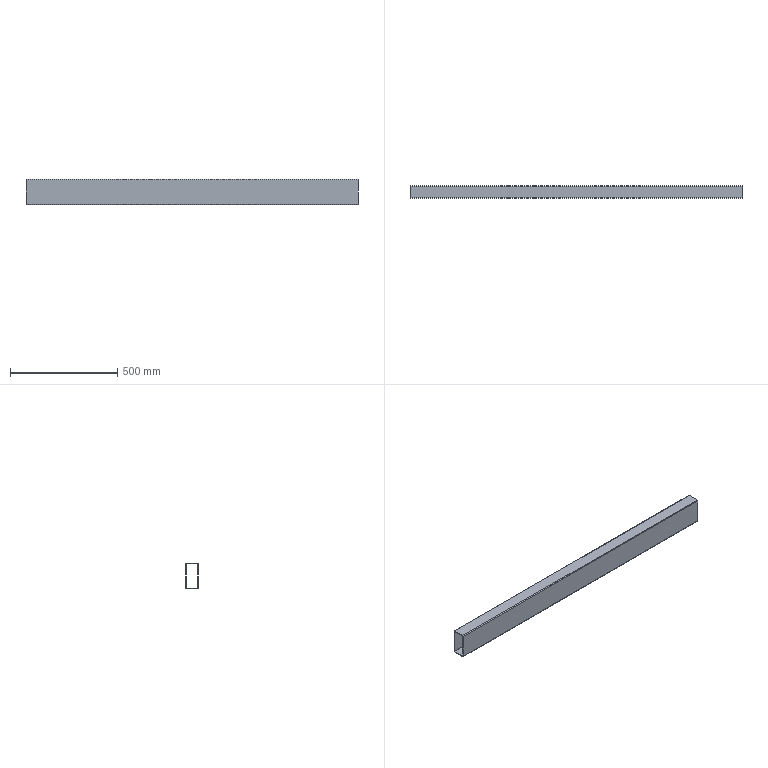Part | SolidWorks | features BaseBody 1 | 1 solid | 18 faces | box 1545 x 60 x 120 mm | volume 1597065 mm3 | plane 10 | cylinder 8 | commonest cylinder face diameters 1 x4 7 x4
STEP:
#1=CARTESIAN_POINT('',(772.5,26.5,-60.));
#2=VERTEX_POINT('',#1);
#3=CARTESIAN_POINT('',(772.5,30.,-56.5));
#4=VERTEX_POINT('',#3);
#5=CARTESIAN_POINT('',(772.5,26.5,-56.5));
#6=DIRECTION('',(1.,0.,0.));
#7=DIRECTION('',(0.,0.,1.));
#8=AXIS2_PLACEMENT_3D('',#5,#6,#7);
#9=CIRCLE('',#8,3.5);
#10=EDGE_CURVE('',#2,#4,#9,.T.);
#11=ORIENTED_EDGE('',*,*,#10,.T.);
#12=CARTESIAN_POINT('',(772.5,30.,56.5));
#13=VERTEX_POINT('',#12);
#14=CARTESIAN_POINT('',(772.5,30.,56.5));
#15=DIRECTION('',(0.,0.,1.));
#16=VECTOR('',#15,1000.);
#17=LINE('',#14,#16);
#18=EDGE_CURVE('',#4,#13,#17,.T.);
#19=ORIENTED_EDGE('',*,*,#18,.T.);
#20=CARTESIAN_POINT('',(772.5,26.5,60.));
#21=VERTEX_POINT('',#20);
#22=CARTESIAN_POINT('',(772.5,26.5,56.5));
#23=DIRECTION('',(1.,0.,0.));
#24=DIRECTION('',(0.,0.,-1.));
#25=AXIS2_PLACEMENT_3D('',#22,#23,#24);
#26=CIRCLE('',#25,3.5);
#27=EDGE_CURVE('',#13,#21,#26,.T.);
#28=ORIENTED_EDGE('',*,*,#27,.T.);
#29=CARTESIAN_POINT('',(772.5,-26.5,60.));
#30=VERTEX_POINT('',#29);
#31=CARTESIAN_POINT('',(772.5,26.5,60.));
#32=DIRECTION('',(0.,-1.,0.));
#33=VECTOR('',#32,1000.);
#34=LINE('',#31,#33);
#35=EDGE_CURVE('',#21,#30,#34,.T.);
#36=ORIENTED_EDGE('',*,*,#35,.T.);
#37=CARTESIAN_POINT('',(772.5,-30.,56.5));
#38=VERTEX_POINT('',#37);
#39=CARTESIAN_POINT('',(772.5,-26.5,56.5));
#40=DIRECTION('',(1.,0.,0.));
#41=DIRECTION('',(0.,0.,-1.));
#42=AXIS2_PLACEMENT_3D('',#39,#40,#41);
#43=CIRCLE('',#42,3.5);
#44=EDGE_CURVE('',#30,#38,#43,.T.);
#45=ORIENTED_EDGE('',*,*,#44,.T.);
#46=CARTESIAN_POINT('',(772.5,-30.,-56.5));
#47=VERTEX_POINT('',#46);
#48=CARTESIAN_POINT('',(772.5,-30.,56.5));
#49=DIRECTION('',(0.,0.,-1.));
#50=VECTOR('',#49,1000.);
#51=LINE('',#48,#50);
#52=EDGE_CURVE('',#38,#47,#51,.T.);
#53=ORIENTED_EDGE('',*,*,#52,.T.);
#54=CARTESIAN_POINT('',(772.5,-26.5,-60.));
#55=VERTEX_POINT('',#54);
#56=CARTESIAN_POINT('',(772.5,-26.5,-56.5));
#57=DIRECTION('',(1.,0.,0.));
#58=DIRECTION('',(0.,0.,-1.));
#59=AXIS2_PLACEMENT_3D('',#56,#57,#58);
#60=CIRCLE('',#59,3.5);
#61=EDGE_CURVE('',#47,#55,#60,.T.);
#62=ORIENTED_EDGE('',*,*,#61,.T.);
#63=CARTESIAN_POINT('',(772.5,26.5,-60.));
#64=DIRECTION('',(0.,1.,0.));
#65=VECTOR('',#64,1000.);
#66=LINE('',#63,#65);
#67=EDGE_CURVE('',#55,#2,#66,.T.);
#68=ORIENTED_EDGE('',*,*,#67,.T.);
#69=EDGE_LOOP('',(#11,#19,#28,#36,#45,#53,#62,#68));
#70=FACE_OUTER_BOUND('',#69,.T.);
#71=CARTESIAN_POINT('',(772.5,27.,-56.5));
#72=VERTEX_POINT('',#71);
#73=CARTESIAN_POINT('',(772.5,27.,56.5));
#74=VERTEX_POINT('',#73);
#75=CARTESIAN_POINT('',(772.5,27.,-56.5));
#76=DIRECTION('',(0.,0.,1.));
#77=VECTOR('',#76,1000.);
#78=LINE('',#75,#77);
#79=EDGE_CURVE('',#72,#74,#78,.T.);
#80=ORIENTED_EDGE('',*,*,#79,.F.);
#81=CARTESIAN_POINT('',(772.5,26.5,-57.));
#82=VERTEX_POINT('',#81);
#83=CARTESIAN_POINT('',(772.5,26.5,-56.5));
#84=DIRECTION('',(1.,0.,0.));
#85=DIRECTION('',(0.,0.,1.));
#86=AXIS2_PLACEMENT_3D('',#83,#84,#85);
#87=CIRCLE('',#86,0.5);
#88=EDGE_CURVE('',#82,#72,#87,.T.);
#89=ORIENTED_EDGE('',*,*,#88,.F.);
#90=CARTESIAN_POINT('',(772.5,-26.5,-57.));
#91=VERTEX_POINT('',#90);
#92=CARTESIAN_POINT('',(772.5,26.5,-57.));
#93=DIRECTION('',(0.,1.,0.));
#94=VECTOR('',#93,1000.);
#95=LINE('',#92,#94);
#96=EDGE_CURVE('',#91,#82,#95,.T.);
#97=ORIENTED_EDGE('',*,*,#96,.F.);
#98=CARTESIAN_POINT('',(772.5,-27.,-56.5));
#99=VERTEX_POINT('',#98);
#100=CARTESIAN_POINT('',(772.5,-26.5,-56.5));
#101=DIRECTION('',(1.,0.,0.));
#102=DIRECTION('',(0.,0.,1.));
#103=AXIS2_PLACEMENT_3D('',#100,#101,#102);
#104=CIRCLE('',#103,0.5);
#105=EDGE_CURVE('',#99,#91,#104,.T.);
#106=ORIENTED_EDGE('',*,*,#105,.F.);
#107=CARTESIAN_POINT('',(772.5,-27.,56.5));
#108=VERTEX_POINT('',#107);
#109=CARTESIAN_POINT('',(772.5,-27.,-56.5));
#110=DIRECTION('',(0.,0.,-1.));
#111=VECTOR('',#110,1000.);
#112=LINE('',#109,#111);
#113=EDGE_CURVE('',#108,#99,#112,.T.);
#114=ORIENTED_EDGE('',*,*,#113,.F.);
#115=CARTESIAN_POINT('',(772.5,-26.5,57.));
#116=VERTEX_POINT('',#115);
#117=CARTESIAN_POINT('',(772.5,-26.5,56.5));
#118=DIRECTION('',(1.,0.,0.));
#119=DIRECTION('',(0.,0.,1.));
#120=AXIS2_PLACEMENT_3D('',#117,#118,#119);
#121=CIRCLE('',#120,0.5);
#122=EDGE_CURVE('',#116,#108,#121,.T.);
#123=ORIENTED_EDGE('',*,*,#122,.F.);
#124=CARTESIAN_POINT('',(772.5,26.5,57.));
#125=VERTEX_POINT('',#124);
#126=CARTESIAN_POINT('',(772.5,26.5,57.));
#127=DIRECTION('',(0.,-1.,0.));
#128=VECTOR('',#127,1000.);
#129=LINE('',#126,#128);
#130=EDGE_CURVE('',#125,#116,#129,.T.);
#131=ORIENTED_EDGE('',*,*,#130,.F.);
#132=CARTESIAN_POINT('',(772.5,26.5,56.5));
#133=DIRECTION('',(1.,0.,0.));
#134=DIRECTION('',(0.,0.,1.));
#135=AXIS2_PLACEMENT_3D('',#132,#133,#134);
#136=CIRCLE('',#135,0.5);
#137=EDGE_CURVE('',#74,#125,#136,.T.);
#138=ORIENTED_EDGE('',*,*,#137,.F.);
#139=EDGE_LOOP('',(#80,#89,#97,#106,#114,#123,#131,#138));
#140=FACE_BOUND('',#139,.T.);
#141=CARTESIAN_POINT('',(772.5,26.5,-56.5));
#142=DIRECTION('',(1.,0.,0.));
#143=DIRECTION('',(0.,0.,-1.));
#144=AXIS2_PLACEMENT_3D('',#141,#142,#143);
#145=PLANE('',#144);
#146=ADVANCED_FACE('',(#70,#140),#145,.T.);
#147=CARTESIAN_POINT('',(-772.5,26.5,-60.));
#148=VERTEX_POINT('',#147);
#149=CARTESIAN_POINT('',(-772.5,30.,-56.5));
#150=VERTEX_POINT('',#149);
#151=CARTESIAN_POINT('',(-772.5,26.5,-56.5));
#152=DIRECTION('',(1.,0.,0.));
#153=DIRECTION('',(0.,0.,1.));
#154=AXIS2_PLACEMENT_3D('',#151,#152,#153);
#155=CIRCLE('',#154,3.5);
#156=EDGE_CURVE('',#148,#150,#155,.T.);
#157=ORIENTED_EDGE('',*,*,#156,.F.);
#158=CARTESIAN_POINT('',(-772.5,-26.5,-60.));
#159=VERTEX_POINT('',#158);
#160=CARTESIAN_POINT('',(-772.5,26.5,-60.));
#161=DIRECTION('',(0.,1.,0.));
#162=VECTOR('',#161,1000.);
#163=LINE('',#160,#162);
#164=EDGE_CURVE('',#159,#148,#163,.T.);
#165=ORIENTED_EDGE('',*,*,#164,.F.);
#166=CARTESIAN_POINT('',(-772.5,-30.,-56.5));
#167=VERTEX_POINT('',#166);
#168=CARTESIAN_POINT('',(-772.5,-26.5,-56.5));
#169=DIRECTION('',(1.,0.,0.));
#170=DIRECTION('',(0.,0.,-1.));
#171=AXIS2_PLACEMENT_3D('',#168,#169,#170);
#172=CIRCLE('',#171,3.5);
#173=EDGE_CURVE('',#167,#159,#172,.T.);
#174=ORIENTED_EDGE('',*,*,#173,.F.);
#175=CARTESIAN_POINT('',(-772.5,-30.,56.5));
#176=VERTEX_POINT('',#175);
#177=CARTESIAN_POINT('',(-772.5,-30.,56.5));
#178=DIRECTION('',(0.,0.,-1.));
#179=VECTOR('',#178,1000.);
#180=LINE('',#177,#179);
#181=EDGE_CURVE('',#176,#167,#180,.T.);
#182=ORIENTED_EDGE('',*,*,#181,.F.);
#183=CARTESIAN_POINT('',(-772.5,-26.5,60.));
#184=VERTEX_POINT('',#183);
#185=CARTESIAN_POINT('',(-772.5,-26.5,56.5));
#186=DIRECTION('',(1.,0.,0.));
#187=DIRECTION('',(0.,0.,-1.));
#188=AXIS2_PLACEMENT_3D('',#185,#186,#187);
#189=CIRCLE('',#188,3.5);
#190=EDGE_CURVE('',#184,#176,#189,.T.);
#191=ORIENTED_EDGE('',*,*,#190,.F.);
#192=CARTESIAN_POINT('',(-772.5,26.5,60.));
#193=VERTEX_POINT('',#192);
#194=CARTESIAN_POINT('',(-772.5,26.5,60.));
#195=DIRECTION('',(0.,-1.,0.));
#196=VECTOR('',#195,1000.);
#197=LINE('',#194,#196);
#198=EDGE_CURVE('',#193,#184,#197,.T.);
#199=ORIENTED_EDGE('',*,*,#198,.F.);
#200=CARTESIAN_POINT('',(-772.5,30.,56.5));
#201=VERTEX_POINT('',#200);
#202=CARTESIAN_POINT('',(-772.5,26.5,56.5));
#203=DIRECTION('',(1.,0.,0.));
#204=DIRECTION('',(0.,0.,-1.));
#205=AXIS2_PLACEMENT_3D('',#202,#203,#204);
#206=CIRCLE('',#205,3.5);
#207=EDGE_CURVE('',#201,#193,#206,.T.);
#208=ORIENTED_EDGE('',*,*,#207,.F.);
#209=CARTESIAN_POINT('',(-772.5,30.,56.5));
#210=DIRECTION('',(0.,0.,1.));
#211=VECTOR('',#210,1000.);
#212=LINE('',#209,#211);
#213=EDGE_CURVE('',#150,#201,#212,.T.);
#214=ORIENTED_EDGE('',*,*,#213,.F.);
#215=EDGE_LOOP('',(#157,#165,#174,#182,#191,#199,#208,#214));
#216=FACE_OUTER_BOUND('',#215,.T.);
#217=CARTESIAN_POINT('',(-772.5,26.5,-57.));
#218=VERTEX_POINT('',#217);
#219=CARTESIAN_POINT('',(-772.5,27.,-56.5));
#220=VERTEX_POINT('',#219);
#221=CARTESIAN_POINT('',(-772.5,26.5,-56.5));
#222=DIRECTION('',(1.,0.,0.));
#223=DIRECTION('',(0.,0.,1.));
#224=AXIS2_PLACEMENT_3D('',#221,#222,#223);
#225=CIRCLE('',#224,0.5);
#226=EDGE_CURVE('',#218,#220,#225,.T.);
#227=ORIENTED_EDGE('',*,*,#226,.T.);
#228=CARTESIAN_POINT('',(-772.5,27.,56.5));
#229=VERTEX_POINT('',#228);
#230=CARTESIAN_POINT('',(-772.5,27.,-56.5));
#231=DIRECTION('',(0.,0.,1.));
#232=VECTOR('',#231,1000.);
#233=LINE('',#230,#232);
#234=EDGE_CURVE('',#220,#229,#233,.T.);
#235=ORIENTED_EDGE('',*,*,#234,.T.);
#236=CARTESIAN_POINT('',(-772.5,26.5,57.));
#237=VERTEX_POINT('',#236);
#238=CARTESIAN_POINT('',(-772.5,26.5,56.5));
#239=DIRECTION('',(1.,0.,0.));
#240=DIRECTION('',(0.,0.,1.));
#241=AXIS2_PLACEMENT_3D('',#238,#239,#240);
#242=CIRCLE('',#241,0.5);
#243=EDGE_CURVE('',#229,#237,#242,.T.);
#244=ORIENTED_EDGE('',*,*,#243,.T.);
#245=CARTESIAN_POINT('',(-772.5,-26.5,57.));
#246=VERTEX_POINT('',#245);
#247=CARTESIAN_POINT('',(-772.5,26.5,57.));
#248=DIRECTION('',(0.,-1.,0.));
#249=VECTOR('',#248,1000.);
#250=LINE('',#247,#249);
#251=EDGE_CURVE('',#237,#246,#250,.T.);
#252=ORIENTED_EDGE('',*,*,#251,.T.);
#253=CARTESIAN_POINT('',(-772.5,-27.,56.5));
#254=VERTEX_POINT('',#253);
#255=CARTESIAN_POINT('',(-772.5,-26.5,56.5));
#256=DIRECTION('',(1.,0.,0.));
#257=DIRECTION('',(0.,0.,1.));
#258=AXIS2_PLACEMENT_3D('',#255,#256,#257);
#259=CIRCLE('',#258,0.5);
#260=EDGE_CURVE('',#246,#254,#259,.T.);
#261=ORIENTED_EDGE('',*,*,#260,.T.);
#262=CARTESIAN_POINT('',(-772.5,-27.,-56.5));
#263=VERTEX_POINT('',#262);
#264=CARTESIAN_POINT('',(-772.5,-27.,-56.5));
#265=DIRECTION('',(0.,0.,-1.));
#266=VECTOR('',#265,1000.);
#267=LINE('',#264,#266);
#268=EDGE_CURVE('',#254,#263,#267,.T.);
#269=ORIENTED_EDGE('',*,*,#268,.T.);
#270=CARTESIAN_POINT('',(-772.5,-26.5,-57.));
#271=VERTEX_POINT('',#270);
#272=CARTESIAN_POINT('',(-772.5,-26.5,-56.5));
#273=DIRECTION('',(1.,0.,0.));
#274=DIRECTION('',(0.,0.,1.));
#275=AXIS2_PLACEMENT_3D('',#272,#273,#274);
#276=CIRCLE('',#275,0.5);
#277=EDGE_CURVE('',#263,#271,#276,.T.);
#278=ORIENTED_EDGE('',*,*,#277,.T.);
#279=CARTESIAN_POINT('',(-772.5,26.5,-57.));
#280=DIRECTION('',(0.,1.,0.));
#281=VECTOR('',#280,1000.);
#282=LINE('',#279,#281);
#283=EDGE_CURVE('',#271,#218,#282,.T.);
#284=ORIENTED_EDGE('',*,*,#283,.T.);
#285=EDGE_LOOP('',(#227,#235,#244,#252,#261,#269,#278,#284));
#286=FACE_BOUND('',#285,.T.);
#287=CARTESIAN_POINT('',(-772.5,26.5,-56.5));
#288=DIRECTION('',(1.,0.,0.));
#289=DIRECTION('',(0.,0.,-1.));
#290=AXIS2_PLACEMENT_3D('',#287,#288,#289);
#291=PLANE('',#290);
#292=ADVANCED_FACE('',(#216,#286),#291,.F.);
#293=ORIENTED_EDGE('',*,*,#156,.T.);
#294=CARTESIAN_POINT('',(772.5,30.,-56.5));
#295=DIRECTION('',(-1.,0.,0.));
#296=VECTOR('',#295,1000.);
#297=LINE('',#294,#296);
#298=EDGE_CURVE('',#4,#150,#297,.T.);
#299=ORIENTED_EDGE('',*,*,#298,.F.);
#300=ORIENTED_EDGE('',*,*,#10,.F.);
#301=CARTESIAN_POINT('',(772.5,26.5,-60.));
#302=DIRECTION('',(-1.,0.,0.));
#303=VECTOR('',#302,1000.);
#304=LINE('',#301,#303);
#305=EDGE_CURVE('',#2,#148,#304,.T.);
#306=ORIENTED_EDGE('',*,*,#305,.T.);
#307=EDGE_LOOP('',(#293,#299,#300,#306));
#308=FACE_OUTER_BOUND('',#307,.T.);
#309=CARTESIAN_POINT('',(772.5,26.5,-56.5));
#310=DIRECTION('',(-1.,0.,0.));
#311=DIRECTION('',(0.,0.,1.));
#312=AXIS2_PLACEMENT_3D('',#309,#310,#311);
#313=CYLINDRICAL_SURFACE('',#312,3.5);
#314=ADVANCED_FACE('',(#308),#313,.T.);
#315=ORIENTED_EDGE('',*,*,#213,.T.);
#316=CARTESIAN_POINT('',(772.5,30.,56.5));
#317=DIRECTION('',(-1.,0.,0.));
#318=VECTOR('',#317,1000.);
#319=LINE('',#316,#318);
#320=EDGE_CURVE('',#13,#201,#319,.T.);
#321=ORIENTED_EDGE('',*,*,#320,.F.);
#322=ORIENTED_EDGE('',*,*,#18,.F.);
#323=ORIENTED_EDGE('',*,*,#298,.T.);
#324=EDGE_LOOP('',(#315,#321,#322,#323));
#325=FACE_OUTER_BOUND('',#324,.T.);
#326=CARTESIAN_POINT('',(772.5,30.,56.5));
#327=DIRECTION('',(0.,-1.,0.));
#328=DIRECTION('',(0.,0.,-1.));
#329=AXIS2_PLACEMENT_3D('',#326,#327,#328);
#330=PLANE('',#329);
#331=ADVANCED_FACE('',(#325),#330,.F.);
#332=ORIENTED_EDGE('',*,*,#207,.T.);
#333=CARTESIAN_POINT('',(772.5,26.5,60.));
#334=DIRECTION('',(-1.,0.,0.));
#335=VECTOR('',#334,1000.);
#336=LINE('',#333,#335);
#337=EDGE_CURVE('',#21,#193,#336,.T.);
#338=ORIENTED_EDGE('',*,*,#337,.F.);
#339=ORIENTED_EDGE('',*,*,#27,.F.);
#340=ORIENTED_EDGE('',*,*,#320,.T.);
#341=EDGE_LOOP('',(#332,#338,#339,#340));
#342=FACE_OUTER_BOUND('',#341,.T.);
#343=CARTESIAN_POINT('',(772.5,26.5,56.5));
#344=DIRECTION('',(-1.,0.,0.));
#345=DIRECTION('',(0.,0.,1.));
#346=AXIS2_PLACEMENT_3D('',#343,#344,#345);
#347=CYLINDRICAL_SURFACE('',#346,3.5);
#348=ADVANCED_FACE('',(#342),#347,.T.);
#349=ORIENTED_EDGE('',*,*,#198,.T.);
#350=CARTESIAN_POINT('',(772.5,-26.5,60.));
#351=DIRECTION('',(-1.,0.,0.));
#352=VECTOR('',#351,1000.);
#353=LINE('',#350,#352);
#354=EDGE_CURVE('',#30,#184,#353,.T.);
#355=ORIENTED_EDGE('',*,*,#354,.F.);
#356=ORIENTED_EDGE('',*,*,#35,.F.);
#357=ORIENTED_EDGE('',*,*,#337,.T.);
#358=EDGE_LOOP('',(#349,#355,#356,#357));
#359=FACE_OUTER_BOUND('',#358,.T.);
#360=CARTESIAN_POINT('',(772.5,26.5,60.));
#361=DIRECTION('',(0.,0.,-1.));
#362=DIRECTION('',(0.,1.,0.));
#363=AXIS2_PLACEMENT_3D('',#360,#361,#362);
#364=PLANE('',#363);
#365=ADVANCED_FACE('',(#359),#364,.F.);
#366=ORIENTED_EDGE('',*,*,#190,.T.);
#367=CARTESIAN_POINT('',(772.5,-30.,56.5));
#368=DIRECTION('',(-1.,0.,0.));
#369=VECTOR('',#368,1000.);
#370=LINE('',#367,#369);
#371=EDGE_CURVE('',#38,#176,#370,.T.);
#372=ORIENTED_EDGE('',*,*,#371,.F.);
#373=ORIENTED_EDGE('',*,*,#44,.F.);
#374=ORIENTED_EDGE('',*,*,#354,.T.);
#375=EDGE_LOOP('',(#366,#372,#373,#374));
#376=FACE_OUTER_BOUND('',#375,.T.);
#377=CARTESIAN_POINT('',(772.5,-26.5,56.5));
#378=DIRECTION('',(-1.,0.,0.));
#379=DIRECTION('',(0.,0.,1.));
#380=AXIS2_PLACEMENT_3D('',#377,#378,#379);
#381=CYLINDRICAL_SURFACE('',#380,3.5);
#382=ADVANCED_FACE('',(#376),#381,.T.);
#383=ORIENTED_EDGE('',*,*,#181,.T.);
#384=CARTESIAN_POINT('',(772.5,-30.,-56.5));
#385=DIRECTION('',(-1.,0.,0.));
#386=VECTOR('',#385,1000.);
#387=LINE('',#384,#386);
#388=EDGE_CURVE('',#47,#167,#387,.T.);
#389=ORIENTED_EDGE('',*,*,#388,.F.);
#390=ORIENTED_EDGE('',*,*,#52,.F.);
#391=ORIENTED_EDGE('',*,*,#371,.T.);
#392=EDGE_LOOP('',(#383,#389,#390,#391));
#393=FACE_OUTER_BOUND('',#392,.T.);
#394=CARTESIAN_POINT('',(772.5,-30.,56.5));
#395=DIRECTION('',(0.,1.,0.));
#396=DIRECTION('',(0.,0.,1.));
#397=AXIS2_PLACEMENT_3D('',#394,#395,#396);
#398=PLANE('',#397);
#399=ADVANCED_FACE('',(#393),#398,.F.);
#400=ORIENTED_EDGE('',*,*,#173,.T.);
#401=CARTESIAN_POINT('',(772.5,-26.5,-60.));
#402=DIRECTION('',(-1.,0.,0.));
#403=VECTOR('',#402,1000.);
#404=LINE('',#401,#403);
#405=EDGE_CURVE('',#55,#159,#404,.T.);
#406=ORIENTED_EDGE('',*,*,#405,.F.);
#407=ORIENTED_EDGE('',*,*,#61,.F.);
#408=ORIENTED_EDGE('',*,*,#388,.T.);
#409=EDGE_LOOP('',(#400,#406,#407,#408));
#410=FACE_OUTER_BOUND('',#409,.T.);
#411=CARTESIAN_POINT('',(772.5,-26.5,-56.5));
#412=DIRECTION('',(-1.,0.,0.));
#413=DIRECTION('',(0.,0.,1.));
#414=AXIS2_PLACEMENT_3D('',#411,#412,#413);
#415=CYLINDRICAL_SURFACE('',#414,3.5);
#416=ADVANCED_FACE('',(#410),#415,.T.);
#417=ORIENTED_EDGE('',*,*,#164,.T.);
#418=ORIENTED_EDGE('',*,*,#305,.F.);
#419=ORIENTED_EDGE('',*,*,#67,.F.);
#420=ORIENTED_EDGE('',*,*,#405,.T.);
#421=EDGE_LOOP('',(#417,#418,#419,#420));
#422=FACE_OUTER_BOUND('',#421,.T.);
#423=CARTESIAN_POINT('',(772.5,26.5,-60.));
#424=DIRECTION('',(0.,0.,1.));
#425=DIRECTION('',(0.,-1.,0.));
#426=AXIS2_PLACEMENT_3D('',#423,#424,#425);
#427=PLANE('',#426);
#428=ADVANCED_FACE('',(#422),#427,.F.);
#429=ORIENTED_EDGE('',*,*,#226,.F.);
#430=CARTESIAN_POINT('',(772.5,26.5,-57.));
#431=DIRECTION('',(-1.,0.,0.));
#432=VECTOR('',#431,1000.);
#433=LINE('',#430,#432);
#434=EDGE_CURVE('',#82,#218,#433,.T.);
#435=ORIENTED_EDGE('',*,*,#434,.F.);
#436=ORIENTED_EDGE('',*,*,#88,.T.);
#437=CARTESIAN_POINT('',(772.5,27.,-56.5));
#438=DIRECTION('',(-1.,0.,0.));
#439=VECTOR('',#438,1000.);
#440=LINE('',#437,#439);
#441=EDGE_CURVE('',#72,#220,#440,.T.);
#442=ORIENTED_EDGE('',*,*,#441,.T.);
#443=EDGE_LOOP('',(#429,#435,#436,#442));
#444=FACE_OUTER_BOUND('',#443,.T.);
#445=CARTESIAN_POINT('',(772.5,26.5,-56.5));
#446=DIRECTION('',(-1.,0.,0.));
#447=DIRECTION('',(0.,0.,1.));
#448=AXIS2_PLACEMENT_3D('',#445,#446,#447);
#449=CYLINDRICAL_SURFACE('',#448,0.5);
#450=ADVANCED_FACE('',(#444),#449,.F.);
#451=ORIENTED_EDGE('',*,*,#234,.F.);
#452=ORIENTED_EDGE('',*,*,#441,.F.);
#453=ORIENTED_EDGE('',*,*,#79,.T.);
#454=CARTESIAN_POINT('',(772.5,27.,56.5));
#455=DIRECTION('',(-1.,0.,0.));
#456=VECTOR('',#455,1000.);
#457=LINE('',#454,#456);
#458=EDGE_CURVE('',#74,#229,#457,.T.);
#459=ORIENTED_EDGE('',*,*,#458,.T.);
#460=EDGE_LOOP('',(#451,#452,#453,#459));
#461=FACE_OUTER_BOUND('',#460,.T.);
#462=CARTESIAN_POINT('',(772.5,27.,-56.5));
#463=DIRECTION('',(0.,-1.,0.));
#464=DIRECTION('',(0.,0.,-1.));
#465=AXIS2_PLACEMENT_3D('',#462,#463,#464);
#466=PLANE('',#465);
#467=ADVANCED_FACE('',(#461),#466,.T.);
#468=ORIENTED_EDGE('',*,*,#243,.F.);
#469=ORIENTED_EDGE('',*,*,#458,.F.);
#470=ORIENTED_EDGE('',*,*,#137,.T.);
#471=CARTESIAN_POINT('',(772.5,26.5,57.));
#472=DIRECTION('',(-1.,0.,0.));
#473=VECTOR('',#472,1000.);
#474=LINE('',#471,#473);
#475=EDGE_CURVE('',#125,#237,#474,.T.);
#476=ORIENTED_EDGE('',*,*,#475,.T.);
#477=EDGE_LOOP('',(#468,#469,#470,#476));
#478=FACE_OUTER_BOUND('',#477,.T.);
#479=CARTESIAN_POINT('',(772.5,26.5,56.5));
#480=DIRECTION('',(-1.,0.,0.));
#481=DIRECTION('',(0.,0.,1.));
#482=AXIS2_PLACEMENT_3D('',#479,#480,#481);
#483=CYLINDRICAL_SURFACE('',#482,0.5);
#484=ADVANCED_FACE('',(#478),#483,.F.);
#485=ORIENTED_EDGE('',*,*,#251,.F.);
#486=ORIENTED_EDGE('',*,*,#475,.F.);
#487=ORIENTED_EDGE('',*,*,#130,.T.);
#488=CARTESIAN_POINT('',(772.5,-26.5,57.));
#489=DIRECTION('',(-1.,0.,0.));
#490=VECTOR('',#489,1000.);
#491=LINE('',#488,#490);
#492=EDGE_CURVE('',#116,#246,#491,.T.);
#493=ORIENTED_EDGE('',*,*,#492,.T.);
#494=EDGE_LOOP('',(#485,#486,#487,#493));
#495=FACE_OUTER_BOUND('',#494,.T.);
#496=CARTESIAN_POINT('',(772.5,26.5,57.));
#497=DIRECTION('',(0.,0.,-1.));
#498=DIRECTION('',(0.,1.,0.));
#499=AXIS2_PLACEMENT_3D('',#496,#497,#498);
#500=PLANE('',#499);
#501=ADVANCED_FACE('',(#495),#500,.T.);
#502=ORIENTED_EDGE('',*,*,#260,.F.);
#503=ORIENTED_EDGE('',*,*,#492,.F.);
#504=ORIENTED_EDGE('',*,*,#122,.T.);
#505=CARTESIAN_POINT('',(772.5,-27.,56.5));
#506=DIRECTION('',(-1.,0.,0.));
#507=VECTOR('',#506,1000.);
#508=LINE('',#505,#507);
#509=EDGE_CURVE('',#108,#254,#508,.T.);
#510=ORIENTED_EDGE('',*,*,#509,.T.);
#511=EDGE_LOOP('',(#502,#503,#504,#510));
#512=FACE_OUTER_BOUND('',#511,.T.);
#513=CARTESIAN_POINT('',(772.5,-26.5,56.5));
#514=DIRECTION('',(-1.,0.,0.));
#515=DIRECTION('',(0.,0.,1.));
#516=AXIS2_PLACEMENT_3D('',#513,#514,#515);
#517=CYLINDRICAL_SURFACE('',#516,0.5);
#518=ADVANCED_FACE('',(#512),#517,.F.);
#519=ORIENTED_EDGE('',*,*,#268,.F.);
#520=ORIENTED_EDGE('',*,*,#509,.F.);
#521=ORIENTED_EDGE('',*,*,#113,.T.);
#522=CARTESIAN_POINT('',(772.5,-27.,-56.5));
#523=DIRECTION('',(-1.,0.,0.));
#524=VECTOR('',#523,1000.);
#525=LINE('',#522,#524);
#526=EDGE_CURVE('',#99,#263,#525,.T.);
#527=ORIENTED_EDGE('',*,*,#526,.T.);
#528=EDGE_LOOP('',(#519,#520,#521,#527));
#529=FACE_OUTER_BOUND('',#528,.T.);
#530=CARTESIAN_POINT('',(772.5,-27.,-56.5));
#531=DIRECTION('',(0.,1.,0.));
#532=DIRECTION('',(0.,0.,1.));
#533=AXIS2_PLACEMENT_3D('',#530,#531,#532);
#534=PLANE('',#533);
#535=ADVANCED_FACE('',(#529),#534,.T.);
#536=ORIENTED_EDGE('',*,*,#277,.F.);
#537=ORIENTED_EDGE('',*,*,#526,.F.);
#538=ORIENTED_EDGE('',*,*,#105,.T.);
#539=CARTESIAN_POINT('',(772.5,-26.5,-57.));
#540=DIRECTION('',(-1.,0.,0.));
#541=VECTOR('',#540,1000.);
#542=LINE('',#539,#541);
#543=EDGE_CURVE('',#91,#271,#542,.T.);
#544=ORIENTED_EDGE('',*,*,#543,.T.);
#545=EDGE_LOOP('',(#536,#537,#538,#544));
#546=FACE_OUTER_BOUND('',#545,.T.);
#547=CARTESIAN_POINT('',(772.5,-26.5,-56.5));
#548=DIRECTION('',(-1.,0.,0.));
#549=DIRECTION('',(0.,0.,1.));
#550=AXIS2_PLACEMENT_3D('',#547,#548,#549);
#551=CYLINDRICAL_SURFACE('',#550,0.5);
#552=ADVANCED_FACE('',(#546),#551,.F.);
#553=ORIENTED_EDGE('',*,*,#283,.F.);
#554=ORIENTED_EDGE('',*,*,#543,.F.);
#555=ORIENTED_EDGE('',*,*,#96,.T.);
#556=ORIENTED_EDGE('',*,*,#434,.T.);
#557=EDGE_LOOP('',(#553,#554,#555,#556));
#558=FACE_OUTER_BOUND('',#557,.T.);
#559=CARTESIAN_POINT('',(772.5,26.5,-57.));
#560=DIRECTION('',(0.,0.,1.));
#561=DIRECTION('',(0.,-1.,0.));
#562=AXIS2_PLACEMENT_3D('',#559,#560,#561);
#563=PLANE('',#562);
#564=ADVANCED_FACE('',(#558),#563,.T.);
#565=CLOSED_SHELL('',(#146,#292,#314,#331,#348,#365,#382,#399,#416,#428,#450,#467,#484,#501,#518,#535,#552,#564));
#566=MANIFOLD_SOLID_BREP('',#565);
#567=CARTESIAN_POINT('',(0.,0.,0.));
#568=DIRECTION('',(0.,0.,1.));
#569=DIRECTION('',(1.,0.,0.));
#570=AXIS2_PLACEMENT_3D('',#567,#568,#569);
#571=(LENGTH_UNIT()NAMED_UNIT(*)SI_UNIT(.MILLI.,.METRE.));
#572=UNCERTAINTY_MEASURE_WITH_UNIT(LENGTH_MEASURE(0.00001),#571,'','');
#573=(NAMED_UNIT(*)PLANE_ANGLE_UNIT()SI_UNIT($,.RADIAN.));
#574=(NAMED_UNIT(*)SI_UNIT($,.STERADIAN.)SOLID_ANGLE_UNIT());
#575=(GEOMETRIC_REPRESENTATION_CONTEXT(3)GLOBAL_UNCERTAINTY_ASSIGNED_CONTEXT((#572))GLOBAL_UNIT_ASSIGNED_CONTEXT((#571,#573,#574))REPRESENTATION_CONTEXT('',''));
#576=ADVANCED_BREP_SHAPE_REPRESENTATION('',(#566,#570),#575);